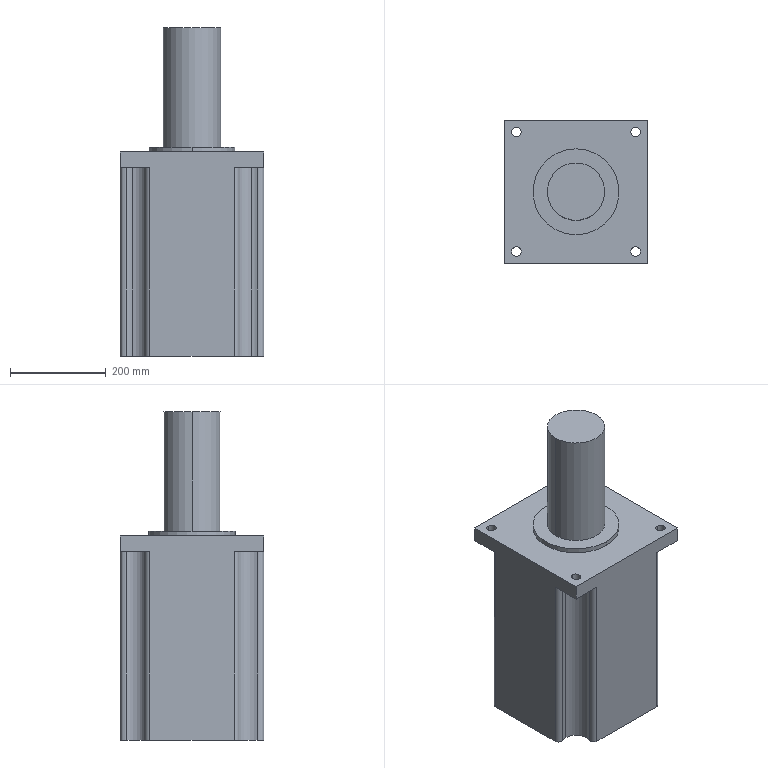Part | SolidWorks | features BaseBody 1, ICE 1, Scale 1 | 1 solid | 40 faces | box 300 x 300 x 687.5 mm | volume 37123455 mm3 | cylinder 28 | plane 12 | commonest cylinder face diameters 20 x18 60 x6 120 x2 180 x2
STEP:
#1=CARTESIAN_POINT('',(2030.017,-675.017,11182.5));
#2=VERTEX_POINT('',#1);
#3=CARTESIAN_POINT('',(1910.017,-675.017,11182.5));
#4=VERTEX_POINT('',#3);
#5=CARTESIAN_POINT('',(1970.017,-675.017,11182.5));
#6=DIRECTION('',(0.,0.,1.));
#7=DIRECTION('',(1.,0.,0.));
#8=AXIS2_PLACEMENT_3D('',#5,#6,#7);
#9=CIRCLE('',#8,60.);
#10=EDGE_CURVE('',#2,#4,#9,.T.);
#11=ORIENTED_EDGE('',*,*,#10,.F.);
#12=CARTESIAN_POINT('',(2030.017,-675.017,10932.5));
#13=VERTEX_POINT('',#12);
#14=CARTESIAN_POINT('',(2030.017,-675.017,11182.5));
#15=DIRECTION('',(0.,0.,-1.));
#16=VECTOR('',#15,1000.);
#17=LINE('',#14,#16);
#18=EDGE_CURVE('',#2,#13,#17,.T.);
#19=ORIENTED_EDGE('',*,*,#18,.T.);
#20=CARTESIAN_POINT('',(1910.017,-675.017,10932.5));
#21=VERTEX_POINT('',#20);
#22=CARTESIAN_POINT('',(1970.017,-675.017,10932.5));
#23=DIRECTION('',(0.,0.,1.));
#24=DIRECTION('',(1.,0.,0.));
#25=AXIS2_PLACEMENT_3D('',#22,#23,#24);
#26=CIRCLE('',#25,60.);
#27=EDGE_CURVE('',#13,#21,#26,.T.);
#28=ORIENTED_EDGE('',*,*,#27,.T.);
#29=CARTESIAN_POINT('',(1910.017,-675.017,11182.5));
#30=DIRECTION('',(0.,0.,-1.));
#31=VECTOR('',#30,1000.);
#32=LINE('',#29,#31);
#33=EDGE_CURVE('',#4,#21,#32,.T.);
#34=ORIENTED_EDGE('',*,*,#33,.F.);
#35=EDGE_LOOP('',(#11,#19,#28,#34));
#36=FACE_OUTER_BOUND('',#35,.T.);
#37=CARTESIAN_POINT('',(1970.017,-675.017,11182.5));
#38=DIRECTION('',(0.,0.,-1.));
#39=DIRECTION('',(-1.,0.,0.));
#40=AXIS2_PLACEMENT_3D('',#37,#38,#39);
#41=CYLINDRICAL_SURFACE('',#40,60.);
#42=ADVANCED_FACE('',(#36),#41,.T.);
#43=CARTESIAN_POINT('',(2106.267,-577.828,10890.));
#44=VERTEX_POINT('',#43);
#45=CARTESIAN_POINT('',(2110.017,-577.098,10890.));
#46=VERTEX_POINT('',#45);
#47=CARTESIAN_POINT('',(2110.017,-587.098,10890.));
#48=DIRECTION('',(0.,0.,-1.));
#49=DIRECTION('',(-1.,0.,0.));
#50=AXIS2_PLACEMENT_3D('',#47,#48,#49);
#51=CIRCLE('',#50,10.);
#52=EDGE_CURVE('',#44,#46,#51,.T.);
#53=ORIENTED_EDGE('',*,*,#52,.T.);
#54=CARTESIAN_POINT('',(2110.017,-577.098,10495.));
#55=VERTEX_POINT('',#54);
#56=CARTESIAN_POINT('',(2110.017,-577.098,10890.));
#57=DIRECTION('',(0.,0.,-1.));
#58=VECTOR('',#57,1000.);
#59=LINE('',#56,#58);
#60=EDGE_CURVE('',#46,#55,#59,.T.);
#61=ORIENTED_EDGE('',*,*,#60,.T.);
#62=CARTESIAN_POINT('',(2106.267,-577.828,10495.));
#63=VERTEX_POINT('',#62);
#64=CARTESIAN_POINT('',(2110.017,-587.098,10495.));
#65=DIRECTION('',(0.,0.,-1.));
#66=DIRECTION('',(-1.,0.,0.));
#67=AXIS2_PLACEMENT_3D('',#64,#65,#66);
#68=CIRCLE('',#67,10.);
#69=EDGE_CURVE('',#63,#55,#68,.T.);
#70=ORIENTED_EDGE('',*,*,#69,.F.);
#71=CARTESIAN_POINT('',(2106.267,-577.828,10890.));
#72=DIRECTION('',(0.,0.,-1.));
#73=VECTOR('',#72,1000.);
#74=LINE('',#71,#73);
#75=EDGE_CURVE('',#44,#63,#74,.T.);
#76=ORIENTED_EDGE('',*,*,#75,.F.);
#77=EDGE_LOOP('',(#53,#61,#70,#76));
#78=FACE_OUTER_BOUND('',#77,.T.);
#79=CARTESIAN_POINT('',(2110.017,-587.098,10890.));
#80=DIRECTION('',(0.,0.,-1.));
#81=DIRECTION('',(0.,1.,0.));
#82=AXIS2_PLACEMENT_3D('',#79,#80,#81);
#83=CYLINDRICAL_SURFACE('',#82,10.);
#84=ADVANCED_FACE('',(#78),#83,.T.);
#85=CARTESIAN_POINT('',(1820.017,-587.098,10890.));
#86=VERTEX_POINT('',#85);
#87=CARTESIAN_POINT('',(1830.017,-577.098,10890.));
#88=VERTEX_POINT('',#87);
#89=CARTESIAN_POINT('',(1830.017,-587.098,10890.));
#90=DIRECTION('',(0.,0.,-1.));
#91=DIRECTION('',(1.,0.,0.));
#92=AXIS2_PLACEMENT_3D('',#89,#90,#91);
#93=CIRCLE('',#92,10.);
#94=EDGE_CURVE('',#86,#88,#93,.T.);
#95=ORIENTED_EDGE('',*,*,#94,.T.);
#96=CARTESIAN_POINT('',(1830.017,-577.098,10495.));
#97=VERTEX_POINT('',#96);
#98=CARTESIAN_POINT('',(1830.017,-577.098,10890.));
#99=DIRECTION('',(0.,0.,-1.));
#100=VECTOR('',#99,1000.);
#101=LINE('',#98,#100);
#102=EDGE_CURVE('',#88,#97,#101,.T.);
#103=ORIENTED_EDGE('',*,*,#102,.T.);
#104=CARTESIAN_POINT('',(1820.017,-587.098,10495.));
#105=VERTEX_POINT('',#104);
#106=CARTESIAN_POINT('',(1830.017,-587.098,10495.));
#107=DIRECTION('',(0.,0.,-1.));
#108=DIRECTION('',(1.,0.,0.));
#109=AXIS2_PLACEMENT_3D('',#106,#107,#108);
#110=CIRCLE('',#109,10.);
#111=EDGE_CURVE('',#105,#97,#110,.T.);
#112=ORIENTED_EDGE('',*,*,#111,.F.);
#113=CARTESIAN_POINT('',(1820.017,-587.098,10890.));
#114=DIRECTION('',(0.,0.,-1.));
#115=VECTOR('',#114,1000.);
#116=LINE('',#113,#115);
#117=EDGE_CURVE('',#86,#105,#116,.T.);
#118=ORIENTED_EDGE('',*,*,#117,.F.);
#119=EDGE_LOOP('',(#95,#103,#112,#118));
#120=FACE_OUTER_BOUND('',#119,.T.);
#121=CARTESIAN_POINT('',(1830.017,-587.098,10890.));
#122=DIRECTION('',(0.,0.,-1.));
#123=DIRECTION('',(0.,1.,0.));
#124=AXIS2_PLACEMENT_3D('',#121,#122,#123);
#125=CYLINDRICAL_SURFACE('',#124,10.);
#126=ADVANCED_FACE('',(#120),#125,.T.);
#127=CARTESIAN_POINT('',(2095.017,-770.017,10890.));
#128=VERTEX_POINT('',#127);
#129=CARTESIAN_POINT('',(2106.267,-772.207,10890.));
#130=VERTEX_POINT('',#129);
#131=CARTESIAN_POINT('',(2095.017,-800.017,10890.));
#132=DIRECTION('',(0.,0.,-1.));
#133=DIRECTION('',(-1.,0.,0.));
#134=AXIS2_PLACEMENT_3D('',#131,#132,#133);
#135=CIRCLE('',#134,30.);
#136=EDGE_CURVE('',#128,#130,#135,.T.);
#137=ORIENTED_EDGE('',*,*,#136,.F.);
#138=CARTESIAN_POINT('',(2095.017,-770.017,10495.));
#139=VERTEX_POINT('',#138);
#140=CARTESIAN_POINT('',(2095.017,-770.017,10890.));
#141=DIRECTION('',(0.,0.,-1.));
#142=VECTOR('',#141,1000.);
#143=LINE('',#140,#142);
#144=EDGE_CURVE('',#128,#139,#143,.T.);
#145=ORIENTED_EDGE('',*,*,#144,.T.);
#146=CARTESIAN_POINT('',(2106.267,-772.207,10495.));
#147=VERTEX_POINT('',#146);
#148=CARTESIAN_POINT('',(2095.017,-800.017,10495.));
#149=DIRECTION('',(0.,0.,-1.));
#150=DIRECTION('',(-1.,0.,0.));
#151=AXIS2_PLACEMENT_3D('',#148,#149,#150);
#152=CIRCLE('',#151,30.);
#153=EDGE_CURVE('',#139,#147,#152,.T.);
#154=ORIENTED_EDGE('',*,*,#153,.T.);
#155=CARTESIAN_POINT('',(2106.267,-772.207,10890.));
#156=DIRECTION('',(0.,0.,-1.));
#157=VECTOR('',#156,1000.);
#158=LINE('',#155,#157);
#159=EDGE_CURVE('',#130,#147,#158,.T.);
#160=ORIENTED_EDGE('',*,*,#159,.F.);
#161=EDGE_LOOP('',(#137,#145,#154,#160));
#162=FACE_OUTER_BOUND('',#161,.T.);
#163=CARTESIAN_POINT('',(2095.017,-800.017,10890.));
#164=DIRECTION('',(0.,0.,-1.));
#165=DIRECTION('',(0.,1.,0.));
#166=AXIS2_PLACEMENT_3D('',#163,#164,#165);
#167=CYLINDRICAL_SURFACE('',#166,30.);
#168=ADVANCED_FACE('',(#162),#167,.F.);
#169=CARTESIAN_POINT('',(1872.828,-811.267,10890.));
#170=VERTEX_POINT('',#169);
#171=CARTESIAN_POINT('',(1845.017,-770.017,10890.));
#172=VERTEX_POINT('',#171);
#173=CARTESIAN_POINT('',(1845.017,-800.017,10890.));
#174=DIRECTION('',(0.,0.,1.));
#175=DIRECTION('',(1.,0.,0.));
#176=AXIS2_PLACEMENT_3D('',#173,#174,#175);
#177=CIRCLE('',#176,30.);
#178=EDGE_CURVE('',#170,#172,#177,.T.);
#179=ORIENTED_EDGE('',*,*,#178,.T.);
#180=CARTESIAN_POINT('',(1845.017,-770.017,10495.));
#181=VERTEX_POINT('',#180);
#182=CARTESIAN_POINT('',(1845.017,-770.017,10890.));
#183=DIRECTION('',(0.,0.,-1.));
#184=VECTOR('',#183,1000.);
#185=LINE('',#182,#184);
#186=EDGE_CURVE('',#172,#181,#185,.T.);
#187=ORIENTED_EDGE('',*,*,#186,.T.);
#188=CARTESIAN_POINT('',(1872.828,-811.267,10495.));
#189=VERTEX_POINT('',#188);
#190=CARTESIAN_POINT('',(1845.017,-800.017,10495.));
#191=DIRECTION('',(0.,0.,1.));
#192=DIRECTION('',(1.,0.,0.));
#193=AXIS2_PLACEMENT_3D('',#190,#191,#192);
#194=CIRCLE('',#193,30.);
#195=EDGE_CURVE('',#189,#181,#194,.T.);
#196=ORIENTED_EDGE('',*,*,#195,.F.);
#197=CARTESIAN_POINT('',(1872.828,-811.267,10890.));
#198=DIRECTION('',(0.,0.,-1.));
#199=VECTOR('',#198,1000.);
#200=LINE('',#197,#199);
#201=EDGE_CURVE('',#170,#189,#200,.T.);
#202=ORIENTED_EDGE('',*,*,#201,.F.);
#203=EDGE_LOOP('',(#179,#187,#196,#202));
#204=FACE_OUTER_BOUND('',#203,.T.);
#205=CARTESIAN_POINT('',(1845.017,-800.017,10890.));
#206=DIRECTION('',(0.,0.,-1.));
#207=DIRECTION('',(0.,1.,0.));
#208=AXIS2_PLACEMENT_3D('',#205,#206,#207);
#209=CYLINDRICAL_SURFACE('',#208,30.);
#210=ADVANCED_FACE('',(#204),#209,.F.);
#211=CARTESIAN_POINT('',(2095.017,-560.017,10922.5));
#212=VERTEX_POINT('',#211);
#213=CARTESIAN_POINT('',(2095.017,-540.017,10922.5));
#214=VERTEX_POINT('',#213);
#215=CARTESIAN_POINT('',(2095.017,-550.017,10922.5));
#216=DIRECTION('',(0.,0.,-1.));
#217=DIRECTION('',(0.,-1.,0.));
#218=AXIS2_PLACEMENT_3D('',#215,#216,#217);
#219=CIRCLE('',#218,10.);
#220=EDGE_CURVE('',#212,#214,#219,.T.);
#221=ORIENTED_EDGE('',*,*,#220,.F.);
#222=CARTESIAN_POINT('',(2095.017,-560.017,10890.));
#223=VERTEX_POINT('',#222);
#224=CARTESIAN_POINT('',(2095.017,-560.017,10995.));
#225=DIRECTION('',(0.,0.,-1.));
#226=VECTOR('',#225,1000.);
#227=LINE('',#224,#226);
#228=EDGE_CURVE('',#212,#223,#227,.T.);
#229=ORIENTED_EDGE('',*,*,#228,.T.);
#230=CARTESIAN_POINT('',(2095.017,-540.017,10890.));
#231=VERTEX_POINT('',#230);
#232=CARTESIAN_POINT('',(2095.017,-550.017,10890.));
#233=DIRECTION('',(0.,0.,1.));
#234=DIRECTION('',(0.,-1.,0.));
#235=AXIS2_PLACEMENT_3D('',#232,#233,#234);
#236=CIRCLE('',#235,10.);
#237=EDGE_CURVE('',#231,#223,#236,.T.);
#238=ORIENTED_EDGE('',*,*,#237,.F.);
#239=CARTESIAN_POINT('',(2095.017,-540.017,10995.));
#240=DIRECTION('',(0.,0.,-1.));
#241=VECTOR('',#240,1000.);
#242=LINE('',#239,#241);
#243=EDGE_CURVE('',#214,#231,#242,.T.);
#244=ORIENTED_EDGE('',*,*,#243,.F.);
#245=EDGE_LOOP('',(#221,#229,#238,#244));
#246=FACE_OUTER_BOUND('',#245,.T.);
#247=CARTESIAN_POINT('',(2095.017,-550.017,10995.));
#248=DIRECTION('',(0.,0.,-1.));
#249=DIRECTION('',(0.,1.,0.));
#250=AXIS2_PLACEMENT_3D('',#247,#248,#249);
#251=CYLINDRICAL_SURFACE('',#250,10.);
#252=ADVANCED_FACE('',(#246),#251,.F.);
#253=CARTESIAN_POINT('',(1970.017,-585.017,10922.5));
#254=VERTEX_POINT('',#253);
#255=CARTESIAN_POINT('',(1970.017,-765.017,10922.5));
#256=VERTEX_POINT('',#255);
#257=CARTESIAN_POINT('',(1970.017,-675.017,10922.5));
#258=DIRECTION('',(0.,0.,1.));
#259=DIRECTION('',(0.,-1.,0.));
#260=AXIS2_PLACEMENT_3D('',#257,#258,#259);
#261=CIRCLE('',#260,90.);
#262=EDGE_CURVE('',#254,#256,#261,.T.);
#263=ORIENTED_EDGE('',*,*,#262,.T.);
#264=CARTESIAN_POINT('',(1970.017,-765.017,10932.5));
#265=VERTEX_POINT('',#264);
#266=CARTESIAN_POINT('',(1970.017,-765.017,10922.5));
#267=DIRECTION('',(0.,0.,1.));
#268=VECTOR('',#267,1000.);
#269=LINE('',#266,#268);
#270=EDGE_CURVE('',#256,#265,#269,.T.);
#271=ORIENTED_EDGE('',*,*,#270,.T.);
#272=CARTESIAN_POINT('',(1970.017,-585.017,10932.5));
#273=VERTEX_POINT('',#272);
#274=CARTESIAN_POINT('',(1970.017,-675.017,10932.5));
#275=DIRECTION('',(0.,0.,-1.));
#276=DIRECTION('',(0.,-1.,0.));
#277=AXIS2_PLACEMENT_3D('',#274,#275,#276);
#278=CIRCLE('',#277,90.);
#279=EDGE_CURVE('',#265,#273,#278,.T.);
#280=ORIENTED_EDGE('',*,*,#279,.T.);
#281=CARTESIAN_POINT('',(1970.017,-585.017,10922.5));
#282=DIRECTION('',(0.,0.,1.));
#283=VECTOR('',#282,1000.);
#284=LINE('',#281,#283);
#285=EDGE_CURVE('',#254,#273,#284,.T.);
#286=ORIENTED_EDGE('',*,*,#285,.F.);
#287=EDGE_LOOP('',(#263,#271,#280,#286));
#288=FACE_OUTER_BOUND('',#287,.T.);
#289=CARTESIAN_POINT('',(1970.017,-675.017,10922.5));
#290=DIRECTION('',(0.,0.,1.));
#291=DIRECTION('',(0.,1.,0.));
#292=AXIS2_PLACEMENT_3D('',#289,#290,#291);
#293=CYLINDRICAL_SURFACE('',#292,90.);
#294=ADVANCED_FACE('',(#288),#293,.T.);
#295=CARTESIAN_POINT('',(1845.017,-810.017,10922.5));
#296=VERTEX_POINT('',#295);
#297=CARTESIAN_POINT('',(1845.017,-790.017,10922.5));
#298=VERTEX_POINT('',#297);
#299=CARTESIAN_POINT('',(1845.017,-800.017,10922.5));
#300=DIRECTION('',(0.,0.,-1.));
#301=DIRECTION('',(0.,-1.,0.));
#302=AXIS2_PLACEMENT_3D('',#299,#300,#301);
#303=CIRCLE('',#302,10.);
#304=EDGE_CURVE('',#296,#298,#303,.T.);
#305=ORIENTED_EDGE('',*,*,#304,.F.);
#306=CARTESIAN_POINT('',(1845.017,-810.017,10890.));
#307=VERTEX_POINT('',#306);
#308=CARTESIAN_POINT('',(1845.017,-810.017,10995.));
#309=DIRECTION('',(0.,0.,-1.));
#310=VECTOR('',#309,1000.);
#311=LINE('',#308,#310);
#312=EDGE_CURVE('',#296,#307,#311,.T.);
#313=ORIENTED_EDGE('',*,*,#312,.T.);
#314=CARTESIAN_POINT('',(1845.017,-790.017,10890.));
#315=VERTEX_POINT('',#314);
#316=CARTESIAN_POINT('',(1845.017,-800.017,10890.));
#317=DIRECTION('',(0.,0.,-1.));
#318=DIRECTION('',(0.,1.,0.));
#319=AXIS2_PLACEMENT_3D('',#316,#317,#318);
#320=CIRCLE('',#319,10.);
#321=EDGE_CURVE('',#307,#315,#320,.T.);
#322=ORIENTED_EDGE('',*,*,#321,.T.);
#323=CARTESIAN_POINT('',(1845.017,-790.017,10995.));
#324=DIRECTION('',(0.,0.,-1.));
#325=VECTOR('',#324,1000.);
#326=LINE('',#323,#325);
#327=EDGE_CURVE('',#298,#315,#326,.T.);
#328=ORIENTED_EDGE('',*,*,#327,.F.);
#329=EDGE_LOOP('',(#305,#313,#322,#328));
#330=FACE_OUTER_BOUND('',#329,.T.);
#331=CARTESIAN_POINT('',(1845.017,-800.017,10995.));
#332=DIRECTION('',(0.,0.,-1.));
#333=DIRECTION('',(0.,1.,0.));
#334=AXIS2_PLACEMENT_3D('',#331,#332,#333);
#335=CYLINDRICAL_SURFACE('',#334,10.);
#336=ADVANCED_FACE('',(#330),#335,.F.);
#337=CARTESIAN_POINT('',(2095.017,-790.017,10922.5));
#338=VERTEX_POINT('',#337);
#339=CARTESIAN_POINT('',(2095.017,-810.017,10922.5));
#340=VERTEX_POINT('',#339);
#341=CARTESIAN_POINT('',(2095.017,-800.017,10922.5));
#342=DIRECTION('',(0.,0.,1.));
#343=DIRECTION('',(0.,-1.,0.));
#344=AXIS2_PLACEMENT_3D('',#341,#342,#343);
#345=CIRCLE('',#344,10.);
#346=EDGE_CURVE('',#338,#340,#345,.T.);
#347=ORIENTED_EDGE('',*,*,#346,.T.);
#348=CARTESIAN_POINT('',(2095.017,-810.017,10890.));
#349=VERTEX_POINT('',#348);
#350=CARTESIAN_POINT('',(2095.017,-810.017,10995.));
#351=DIRECTION('',(0.,0.,-1.));
#352=VECTOR('',#351,1000.);
#353=LINE('',#350,#352);
#354=EDGE_CURVE('',#340,#349,#353,.T.);
#355=ORIENTED_EDGE('',*,*,#354,.T.);
#356=CARTESIAN_POINT('',(2095.017,-790.017,10890.));
#357=VERTEX_POINT('',#356);
#358=CARTESIAN_POINT('',(2095.017,-800.017,10890.));
#359=DIRECTION('',(0.,0.,1.));
#360=DIRECTION('',(0.,1.,0.));
#361=AXIS2_PLACEMENT_3D('',#358,#359,#360);
#362=CIRCLE('',#361,10.);
#363=EDGE_CURVE('',#357,#349,#362,.T.);
#364=ORIENTED_EDGE('',*,*,#363,.F.);
#365=CARTESIAN_POINT('',(2095.017,-790.017,10995.));
#366=DIRECTION('',(0.,0.,-1.));
#367=VECTOR('',#366,1000.);
#368=LINE('',#365,#367);
#369=EDGE_CURVE('',#338,#357,#368,.T.);
#370=ORIENTED_EDGE('',*,*,#369,.F.);
#371=EDGE_LOOP('',(#347,#355,#364,#370));
#372=FACE_OUTER_BOUND('',#371,.T.);
#373=CARTESIAN_POINT('',(2095.017,-800.017,10995.));
#374=DIRECTION('',(0.,0.,-1.));
#375=DIRECTION('',(0.,1.,0.));
#376=AXIS2_PLACEMENT_3D('',#373,#374,#375);
#377=CYLINDRICAL_SURFACE('',#376,10.);
#378=ADVANCED_FACE('',(#372),#377,.F.);
#379=CARTESIAN_POINT('',(1845.017,-560.017,10922.5));
#380=VERTEX_POINT('',#379);
#381=CARTESIAN_POINT('',(1845.017,-540.017,10922.5));
#382=VERTEX_POINT('',#381);
#383=CARTESIAN_POINT('',(1845.017,-550.017,10922.5));
#384=DIRECTION('',(0.,0.,-1.));
#385=DIRECTION('',(0.,-1.,0.));
#386=AXIS2_PLACEMENT_3D('',#383,#384,#385);
#387=CIRCLE('',#386,10.);
#388=EDGE_CURVE('',#380,#382,#387,.T.);
#389=ORIENTED_EDGE('',*,*,#388,.F.);
#390=CARTESIAN_POINT('',(1845.017,-560.017,10890.));
#391=VERTEX_POINT('',#390);
#392=CARTESIAN_POINT('',(1845.017,-560.017,10995.));
#393=DIRECTION('',(0.,0.,-1.));
#394=VECTOR('',#393,1000.);
#395=LINE('',#392,#394);
#396=EDGE_CURVE('',#380,#391,#395,.T.);
#397=ORIENTED_EDGE('',*,*,#396,.T.);
#398=CARTESIAN_POINT('',(1845.017,-540.017,10890.));
#399=VERTEX_POINT('',#398);
#400=CARTESIAN_POINT('',(1845.017,-550.017,10890.));
#401=DIRECTION('',(0.,0.,-1.));
#402=DIRECTION('',(0.,1.,0.));
#403=AXIS2_PLACEMENT_3D('',#400,#401,#402);
#404=CIRCLE('',#403,10.);
#405=EDGE_CURVE('',#391,#399,#404,.T.);
#406=ORIENTED_EDGE('',*,*,#405,.T.);
#407=CARTESIAN_POINT('',(1845.017,-540.017,10995.));
#408=DIRECTION('',(0.,0.,-1.));
#409=VECTOR('',#408,1000.);
#410=LINE('',#407,#409);
#411=EDGE_CURVE('',#382,#399,#410,.T.);
#412=ORIENTED_EDGE('',*,*,#411,.F.);
#413=EDGE_LOOP('',(#389,#397,#406,#412));
#414=FACE_OUTER_BOUND('',#413,.T.);
#415=CARTESIAN_POINT('',(1845.017,-550.017,10995.));
#416=DIRECTION('',(0.,0.,-1.));
#417=DIRECTION('',(0.,1.,0.));
#418=AXIS2_PLACEMENT_3D('',#415,#416,#417);
#419=CYLINDRICAL_SURFACE('',#418,10.);
#420=ADVANCED_FACE('',(#414),#419,.F.);
#421=CARTESIAN_POINT('',(1970.017,-675.017,10932.5));
#422=DIRECTION('',(0.,0.,1.));
#423=DIRECTION('',(1.,0.,0.));
#424=AXIS2_PLACEMENT_3D('',#421,#422,#423);
#425=CIRCLE('',#424,60.);
#426=EDGE_CURVE('',#21,#13,#425,.T.);
#427=ORIENTED_EDGE('',*,*,#426,.F.);
#428=ORIENTED_EDGE('',*,*,#27,.F.);
#429=EDGE_LOOP('',(#427,#428));
#430=FACE_BOUND('',#429,.T.);
#431=CARTESIAN_POINT('',(1970.017,-675.017,10932.5));
#432=DIRECTION('',(0.,0.,-1.));
#433=DIRECTION('',(0.,-1.,0.));
#434=AXIS2_PLACEMENT_3D('',#431,#432,#433);
#435=CIRCLE('',#434,90.);
#436=EDGE_CURVE('',#273,#265,#435,.T.);
#437=ORIENTED_EDGE('',*,*,#436,.F.);
#438=ORIENTED_EDGE('',*,*,#279,.F.);
#439=EDGE_LOOP('',(#437,#438));
#440=FACE_OUTER_BOUND('',#439,.T.);
#441=CARTESIAN_POINT('',(1970.017,-675.017,10932.5));
#442=DIRECTION('',(0.,0.,1.));
#443=DIRECTION('',(0.,1.,0.));
#444=AXIS2_PLACEMENT_3D('',#441,#442,#443);
#445=PLANE('',#444);
#446=ADVANCED_FACE('',(#430,#440),#445,.T.);
#447=CARTESIAN_POINT('',(2067.207,-538.767,10495.));
#448=VERTEX_POINT('',#447);
#449=CARTESIAN_POINT('',(2095.017,-550.017,10495.));
#450=DIRECTION('',(0.,0.,1.));
#451=DIRECTION('',(-1.,0.,0.));
#452=AXIS2_PLACEMENT_3D('',#449,#450,#451);
#453=CIRCLE('',#452,30.);
#454=EDGE_CURVE('',#448,#63,#453,.T.);
#455=ORIENTED_EDGE('',*,*,#454,.T.);
#456=ORIENTED_EDGE('',*,*,#69,.T.);
#457=CARTESIAN_POINT('',(2120.017,-587.098,10495.));
#458=VERTEX_POINT('',#457);
#459=CARTESIAN_POINT('',(2110.017,-587.098,10495.));
#460=DIRECTION('',(0.,0.,-1.));
#461=DIRECTION('',(-1.,0.,0.));
#462=AXIS2_PLACEMENT_3D('',#459,#460,#461);
#463=CIRCLE('',#462,10.);
#464=EDGE_CURVE('',#55,#458,#463,.T.);
#465=ORIENTED_EDGE('',*,*,#464,.T.);
#466=CARTESIAN_POINT('',(2120.017,-762.936,10495.));
#467=VERTEX_POINT('',#466);
#468=CARTESIAN_POINT('',(2120.017,-525.017,10495.));
#469=DIRECTION('',(0.,-1.,0.));
#470=VECTOR('',#469,1000.);
#471=LINE('',#468,#470);
#472=EDGE_CURVE('',#458,#467,#471,.T.);
#473=ORIENTED_EDGE('',*,*,#472,.T.);
#474=CARTESIAN_POINT('',(2110.017,-762.936,10495.));
#475=DIRECTION('',(0.,0.,1.));
#476=DIRECTION('',(-1.,0.,0.));
#477=AXIS2_PLACEMENT_3D('',#474,#475,#476);
#478=CIRCLE('',#477,10.);
#479=EDGE_CURVE('',#147,#467,#478,.T.);
#480=ORIENTED_EDGE('',*,*,#479,.F.);
#481=ORIENTED_EDGE('',*,*,#153,.F.);
#482=CARTESIAN_POINT('',(2067.207,-811.267,10495.));
#483=VERTEX_POINT('',#482);
#484=CARTESIAN_POINT('',(2095.017,-800.017,10495.));
#485=DIRECTION('',(0.,0.,-1.));
#486=DIRECTION('',(-1.,0.,0.));
#487=AXIS2_PLACEMENT_3D('',#484,#485,#486);
#488=CIRCLE('',#487,30.);
#489=EDGE_CURVE('',#483,#139,#488,.T.);
#490=ORIENTED_EDGE('',*,*,#489,.F.);
#491=CARTESIAN_POINT('',(2057.936,-825.017,10495.));
#492=VERTEX_POINT('',#491);
#493=CARTESIAN_POINT('',(2057.936,-815.017,10495.));
#494=DIRECTION('',(0.,0.,1.));
#495=DIRECTION('',(-1.,0.,0.));
#496=AXIS2_PLACEMENT_3D('',#493,#494,#495);
#497=CIRCLE('',#496,10.);
#498=EDGE_CURVE('',#492,#483,#497,.T.);
#499=ORIENTED_EDGE('',*,*,#498,.F.);
#500=CARTESIAN_POINT('',(1882.098,-825.017,10495.));
#501=VERTEX_POINT('',#500);
#502=CARTESIAN_POINT('',(1970.017,-825.017,10495.));
#503=DIRECTION('',(-1.,0.,0.));
#504=VECTOR('',#503,1000.);
#505=LINE('',#502,#504);
#506=EDGE_CURVE('',#492,#501,#505,.T.);
#507=ORIENTED_EDGE('',*,*,#506,.T.);
#508=CARTESIAN_POINT('',(1882.098,-815.017,10495.));
#509=DIRECTION('',(0.,0.,-1.));
#510=DIRECTION('',(1.,0.,0.));
#511=AXIS2_PLACEMENT_3D('',#508,#509,#510);
#512=CIRCLE('',#511,10.);
#513=EDGE_CURVE('',#501,#189,#512,.T.);
#514=ORIENTED_EDGE('',*,*,#513,.T.);
#515=ORIENTED_EDGE('',*,*,#195,.T.);
#516=CARTESIAN_POINT('',(1833.767,-772.207,10495.));
#517=VERTEX_POINT('',#516);
#518=CARTESIAN_POINT('',(1845.017,-800.017,10495.));
#519=DIRECTION('',(0.,0.,1.));
#520=DIRECTION('',(1.,0.,0.));
#521=AXIS2_PLACEMENT_3D('',#518,#519,#520);
#522=CIRCLE('',#521,30.);
#523=EDGE_CURVE('',#181,#517,#522,.T.);
#524=ORIENTED_EDGE('',*,*,#523,.T.);
#525=CARTESIAN_POINT('',(1820.017,-762.936,10495.));
#526=VERTEX_POINT('',#525);
#527=CARTESIAN_POINT('',(1830.017,-762.936,10495.));
#528=DIRECTION('',(0.,0.,-1.));
#529=DIRECTION('',(1.,0.,0.));
#530=AXIS2_PLACEMENT_3D('',#527,#528,#529);
#531=CIRCLE('',#530,10.);
#532=EDGE_CURVE('',#517,#526,#531,.T.);
#533=ORIENTED_EDGE('',*,*,#532,.T.);
#534=CARTESIAN_POINT('',(1820.017,-525.017,10495.));
#535=DIRECTION('',(0.,-1.,0.));
#536=VECTOR('',#535,1000.);
#537=LINE('',#534,#536);
#538=EDGE_CURVE('',#105,#526,#537,.T.);
#539=ORIENTED_EDGE('',*,*,#538,.F.);
#540=ORIENTED_EDGE('',*,*,#111,.T.);
#541=CARTESIAN_POINT('',(1833.767,-577.828,10495.));
#542=VERTEX_POINT('',#541);
#543=CARTESIAN_POINT('',(1830.017,-587.098,10495.));
#544=DIRECTION('',(0.,0.,-1.));
#545=DIRECTION('',(1.,0.,0.));
#546=AXIS2_PLACEMENT_3D('',#543,#544,#545);
#547=CIRCLE('',#546,10.);
#548=EDGE_CURVE('',#97,#542,#547,.T.);
#549=ORIENTED_EDGE('',*,*,#548,.T.);
#550=CARTESIAN_POINT('',(1872.828,-538.767,10495.));
#551=VERTEX_POINT('',#550);
#552=CARTESIAN_POINT('',(1845.017,-550.017,10495.));
#553=DIRECTION('',(0.,0.,1.));
#554=DIRECTION('',(1.,0.,0.));
#555=AXIS2_PLACEMENT_3D('',#552,#553,#554);
#556=CIRCLE('',#555,30.);
#557=EDGE_CURVE('',#542,#551,#556,.T.);
#558=ORIENTED_EDGE('',*,*,#557,.T.);
#559=CARTESIAN_POINT('',(1882.098,-525.017,10495.));
#560=VERTEX_POINT('',#559);
#561=CARTESIAN_POINT('',(1882.098,-535.017,10495.));
#562=DIRECTION('',(0.,0.,-1.));
#563=DIRECTION('',(1.,0.,0.));
#564=AXIS2_PLACEMENT_3D('',#561,#562,#563);
#565=CIRCLE('',#564,10.);
#566=EDGE_CURVE('',#551,#560,#565,.T.);
#567=ORIENTED_EDGE('',*,*,#566,.T.);
#568=CARTESIAN_POINT('',(2057.936,-525.017,10495.));
#569=VERTEX_POINT('',#568);
#570=CARTESIAN_POINT('',(1970.017,-525.017,10495.));
#571=DIRECTION('',(1.,0.,0.));
#572=VECTOR('',#571,1000.);
#573=LINE('',#570,#572);
#574=EDGE_CURVE('',#560,#569,#573,.T.);
#575=ORIENTED_EDGE('',*,*,#574,.T.);
#576=CARTESIAN_POINT('',(2057.936,-535.017,10495.));
#577=DIRECTION('',(0.,0.,-1.));
#578=DIRECTION('',(-1.,0.,0.));
#579=AXIS2_PLACEMENT_3D('',#576,#577,#578);
#580=CIRCLE('',#579,10.);
#581=EDGE_CURVE('',#569,#448,#580,.T.);
#582=ORIENTED_EDGE('',*,*,#581,.T.);
#583=EDGE_LOOP('',(#455,#456,#465,#473,#480,#481,#490,#499,#507,#514,#515,#524,#533,#539,#540,#549,#558,#567,#575,#582));
#584=FACE_OUTER_BOUND('',#583,.T.);
#585=CARTESIAN_POINT('',(1970.017,-525.017,10495.));
#586=DIRECTION('',(0.,0.,-1.));
#587=DIRECTION('',(0.,-1.,0.));
#588=AXIS2_PLACEMENT_3D('',#585,#586,#587);
#589=PLANE('',#588);
#590=ADVANCED_FACE('',(#584),#589,.T.);
#591=CARTESIAN_POINT('',(2120.017,-525.017,10890.));
#592=VERTEX_POINT('',#591);
#593=CARTESIAN_POINT('',(2057.936,-525.017,10890.));
#594=VERTEX_POINT('',#593);
#595=CARTESIAN_POINT('',(2120.017,-525.017,10890.));
#596=DIRECTION('',(-1.,0.,0.));
#597=VECTOR('',#596,1000.);
#598=LINE('',#595,#597);
#599=EDGE_CURVE('',#592,#594,#598,.T.);
#600=ORIENTED_EDGE('',*,*,#599,.T.);
#601=CARTESIAN_POINT('',(2057.936,-525.017,10890.));
#602=DIRECTION('',(0.,0.,-1.));
#603=VECTOR('',#602,1000.);
#604=LINE('',#601,#603);
#605=EDGE_CURVE('',#594,#569,#604,.T.);
#606=ORIENTED_EDGE('',*,*,#605,.T.);
#607=ORIENTED_EDGE('',*,*,#574,.F.);
#608=CARTESIAN_POINT('',(1882.098,-525.017,10890.));
#609=VERTEX_POINT('',#608);
#610=CARTESIAN_POINT('',(1882.098,-525.017,10890.));
#611=DIRECTION('',(0.,0.,-1.));
#612=VECTOR('',#611,1000.);
#613=LINE('',#610,#612);
#614=EDGE_CURVE('',#609,#560,#613,.T.);
#615=ORIENTED_EDGE('',*,*,#614,.F.);
#616=CARTESIAN_POINT('',(1820.017,-525.017,10890.));
#617=VERTEX_POINT('',#616);
#618=CARTESIAN_POINT('',(1882.098,-525.017,10890.));
#619=DIRECTION('',(-1.,0.,0.));
#620=VECTOR('',#619,1000.);
#621=LINE('',#618,#620);
#622=EDGE_CURVE('',#609,#617,#621,.T.);
#623=ORIENTED_EDGE('',*,*,#622,.T.);
#624=CARTESIAN_POINT('',(1820.017,-525.017,10922.5));
#625=VERTEX_POINT('',#624);
#626=CARTESIAN_POINT('',(1820.017,-525.017,10708.75));
#627=DIRECTION('',(0.,0.,-1.));
#628=VECTOR('',#627,1000.);
#629=LINE('',#626,#628);
#630=EDGE_CURVE('',#625,#617,#629,.T.);
#631=ORIENTED_EDGE('',*,*,#630,.F.);
#632=CARTESIAN_POINT('',(2120.017,-525.017,10922.5));
#633=VERTEX_POINT('',#632);
#634=CARTESIAN_POINT('',(1970.017,-525.017,10922.5));
#635=DIRECTION('',(-1.,0.,0.));
#636=VECTOR('',#635,1000.);
#637=LINE('',#634,#636);
#638=EDGE_CURVE('',#633,#625,#637,.T.);
#639=ORIENTED_EDGE('',*,*,#638,.F.);
#640=CARTESIAN_POINT('',(2120.017,-525.017,10708.75));
#641=DIRECTION('',(0.,0.,1.));
#642=VECTOR('',#641,1000.);
#643=LINE('',#640,#642);
#644=EDGE_CURVE('',#592,#633,#643,.T.);
#645=ORIENTED_EDGE('',*,*,#644,.F.);
#646=EDGE_LOOP('',(#600,#606,#607,#615,#623,#631,#639,#645));
#647=FACE_OUTER_BOUND('',#646,.T.);
#648=CARTESIAN_POINT('',(1970.017,-525.017,10708.75));
#649=DIRECTION('',(0.,1.,0.));
#650=DIRECTION('',(1.,0.,0.));
#651=AXIS2_PLACEMENT_3D('',#648,#649,#650);
#652=PLANE('',#651);
#653=ADVANCED_FACE('',(#647),#652,.T.);
#654=CARTESIAN_POINT('',(1820.017,-525.017,10890.));
#655=DIRECTION('',(0.,-1.,0.));
#656=VECTOR('',#655,1000.);
#657=LINE('',#654,#656);
#658=EDGE_CURVE('',#617,#86,#657,.T.);
#659=ORIENTED_EDGE('',*,*,#658,.T.);
#660=ORIENTED_EDGE('',*,*,#117,.T.);
#661=ORIENTED_EDGE('',*,*,#538,.T.);
#662=CARTESIAN_POINT('',(1820.017,-762.936,10890.));
#663=VERTEX_POINT('',#662);
#664=CARTESIAN_POINT('',(1820.017,-762.936,10890.));
#665=DIRECTION('',(0.,0.,-1.));
#666=VECTOR('',#665,1000.);
#667=LINE('',#664,#666);
#668=EDGE_CURVE('',#663,#526,#667,.T.);
#669=ORIENTED_EDGE('',*,*,#668,.F.);
#670=CARTESIAN_POINT('',(1820.017,-825.017,10890.));
#671=VERTEX_POINT('',#670);
#672=CARTESIAN_POINT('',(1820.017,-762.936,10890.));
#673=DIRECTION('',(0.,-1.,0.));
#674=VECTOR('',#673,1000.);
#675=LINE('',#672,#674);
#676=EDGE_CURVE('',#663,#671,#675,.T.);
#677=ORIENTED_EDGE('',*,*,#676,.T.);
#678=CARTESIAN_POINT('',(1820.017,-825.017,10922.5));
#679=VERTEX_POINT('',#678);
#680=CARTESIAN_POINT('',(1820.017,-825.017,10708.75));
#681=DIRECTION('',(0.,0.,1.));
#682=VECTOR('',#681,1000.);
#683=LINE('',#680,#682);
#684=EDGE_CURVE('',#671,#679,#683,.T.);
#685=ORIENTED_EDGE('',*,*,#684,.T.);
#686=CARTESIAN_POINT('',(1820.017,-525.017,10922.5));
#687=DIRECTION('',(0.,-1.,0.));
#688=VECTOR('',#687,1000.);
#689=LINE('',#686,#688);
#690=EDGE_CURVE('',#625,#679,#689,.T.);
#691=ORIENTED_EDGE('',*,*,#690,.F.);
#692=ORIENTED_EDGE('',*,*,#630,.T.);
#693=EDGE_LOOP('',(#659,#660,#661,#669,#677,#685,#691,#692));
#694=FACE_OUTER_BOUND('',#693,.T.);
#695=CARTESIAN_POINT('',(1820.017,-525.017,10708.75));
#696=DIRECTION('',(-1.,0.,0.));
#697=DIRECTION('',(0.,1.,0.));
#698=AXIS2_PLACEMENT_3D('',#695,#696,#697);
#699=PLANE('',#698);
#700=ADVANCED_FACE('',(#694),#699,.T.);
#701=ORIENTED_EDGE('',*,*,#396,.F.);
#702=CARTESIAN_POINT('',(1845.017,-550.017,10922.5));
#703=DIRECTION('',(0.,0.,-1.));
#704=DIRECTION('',(0.,-1.,0.));
#705=AXIS2_PLACEMENT_3D('',#702,#703,#704);
#706=CIRCLE('',#705,10.);
#707=EDGE_CURVE('',#382,#380,#706,.T.);
#708=ORIENTED_EDGE('',*,*,#707,.F.);
#709=ORIENTED_EDGE('',*,*,#411,.T.);
#710=CARTESIAN_POINT('',(1845.017,-550.017,10890.));
#711=DIRECTION('',(0.,0.,-1.));
#712=DIRECTION('',(0.,1.,0.));
#713=AXIS2_PLACEMENT_3D('',#710,#711,#712);
#714=CIRCLE('',#713,10.);
#715=EDGE_CURVE('',#399,#391,#714,.T.);
#716=ORIENTED_EDGE('',*,*,#715,.T.);
#717=EDGE_LOOP('',(#701,#708,#709,#716));
#718=FACE_OUTER_BOUND('',#717,.T.);
#719=CARTESIAN_POINT('',(1845.017,-550.017,10995.));
#720=DIRECTION('',(0.,0.,-1.));
#721=DIRECTION('',(0.,1.,0.));
#722=AXIS2_PLACEMENT_3D('',#719,#720,#721);
#723=CYLINDRICAL_SURFACE('',#722,10.);
#724=ADVANCED_FACE('',(#718),#723,.F.);
#725=ORIENTED_EDGE('',*,*,#506,.F.);
#726=CARTESIAN_POINT('',(2057.936,-825.017,10890.));
#727=VERTEX_POINT('',#726);
#728=CARTESIAN_POINT('',(2057.936,-825.017,10890.));
#729=DIRECTION('',(0.,0.,-1.));
#730=VECTOR('',#729,1000.);
#731=LINE('',#728,#730);
#732=EDGE_CURVE('',#727,#492,#731,.T.);
#733=ORIENTED_EDGE('',*,*,#732,.F.);
#734=CARTESIAN_POINT('',(2120.017,-825.017,10890.));
#735=VERTEX_POINT('',#734);
#736=CARTESIAN_POINT('',(2120.017,-825.017,10890.));
#737=DIRECTION('',(-1.,0.,0.));
#738=VECTOR('',#737,1000.);
#739=LINE('',#736,#738);
#740=EDGE_CURVE('',#735,#727,#739,.T.);
#741=ORIENTED_EDGE('',*,*,#740,.F.);
#742=CARTESIAN_POINT('',(2120.017,-825.017,10922.5));
#743=VERTEX_POINT('',#742);
#744=CARTESIAN_POINT('',(2120.017,-825.017,10708.75));
#745=DIRECTION('',(0.,0.,-1.));
#746=VECTOR('',#745,1000.);
#747=LINE('',#744,#746);
#748=EDGE_CURVE('',#743,#735,#747,.T.);
#749=ORIENTED_EDGE('',*,*,#748,.F.);
#750=CARTESIAN_POINT('',(1970.017,-825.017,10922.5));
#751=DIRECTION('',(1.,0.,0.));
#752=VECTOR('',#751,1000.);
#753=LINE('',#750,#752);
#754=EDGE_CURVE('',#679,#743,#753,.T.);
#755=ORIENTED_EDGE('',*,*,#754,.F.);
#756=ORIENTED_EDGE('',*,*,#684,.F.);
#757=CARTESIAN_POINT('',(1882.098,-825.017,10890.));
#758=VERTEX_POINT('',#757);
#759=CARTESIAN_POINT('',(1820.017,-825.017,10890.));
#760=DIRECTION('',(1.,0.,0.));
#761=VECTOR('',#760,1000.);
#762=LINE('',#759,#761);
#763=EDGE_CURVE('',#671,#758,#762,.T.);
#764=ORIENTED_EDGE('',*,*,#763,.T.);
#765=CARTESIAN_POINT('',(1882.098,-825.017,10890.));
#766=DIRECTION('',(0.,0.,-1.));
#767=VECTOR('',#766,1000.);
#768=LINE('',#765,#767);
#769=EDGE_CURVE('',#758,#501,#768,.T.);
#770=ORIENTED_EDGE('',*,*,#769,.T.);
#771=EDGE_LOOP('',(#725,#733,#741,#749,#755,#756,#764,#770));
#772=FACE_OUTER_BOUND('',#771,.T.);
#773=CARTESIAN_POINT('',(1970.017,-825.017,10708.75));
#774=DIRECTION('',(0.,-1.,0.));
#775=DIRECTION('',(-1.,0.,0.));
#776=AXIS2_PLACEMENT_3D('',#773,#774,#775);
#777=PLANE('',#776);
#778=ADVANCED_FACE('',(#772),#777,.T.);
#779=ORIENTED_EDGE('',*,*,#354,.F.);
#780=CARTESIAN_POINT('',(2095.017,-800.017,10922.5));
#781=DIRECTION('',(0.,0.,1.));
#782=DIRECTION('',(0.,-1.,0.));
#783=AXIS2_PLACEMENT_3D('',#780,#781,#782);
#784=CIRCLE('',#783,10.);
#785=EDGE_CURVE('',#340,#338,#784,.T.);
#786=ORIENTED_EDGE('',*,*,#785,.T.);
#787=ORIENTED_EDGE('',*,*,#369,.T.);
#788=CARTESIAN_POINT('',(2095.017,-800.017,10890.));
#789=DIRECTION('',(0.,0.,1.));
#790=DIRECTION('',(0.,1.,0.));
#791=AXIS2_PLACEMENT_3D('',#788,#789,#790);
#792=CIRCLE('',#791,10.);
#793=EDGE_CURVE('',#349,#357,#792,.T.);
#794=ORIENTED_EDGE('',*,*,#793,.F.);
#795=EDGE_LOOP('',(#779,#786,#787,#794));
#796=FACE_OUTER_BOUND('',#795,.T.);
#797=CARTESIAN_POINT('',(2095.017,-800.017,10995.));
#798=DIRECTION('',(0.,0.,-1.));
#799=DIRECTION('',(0.,1.,0.));
#800=AXIS2_PLACEMENT_3D('',#797,#798,#799);
#801=CYLINDRICAL_SURFACE('',#800,10.);
#802=ADVANCED_FACE('',(#796),#801,.F.);
#803=ORIENTED_EDGE('',*,*,#312,.F.);
#804=CARTESIAN_POINT('',(1845.017,-800.017,10922.5));
#805=DIRECTION('',(0.,0.,-1.));
#806=DIRECTION('',(0.,-1.,0.));
#807=AXIS2_PLACEMENT_3D('',#804,#805,#806);
#808=CIRCLE('',#807,10.);
#809=EDGE_CURVE('',#298,#296,#808,.T.);
#810=ORIENTED_EDGE('',*,*,#809,.F.);
#811=ORIENTED_EDGE('',*,*,#327,.T.);
#812=CARTESIAN_POINT('',(1845.017,-800.017,10890.));
#813=DIRECTION('',(0.,0.,-1.));
#814=DIRECTION('',(0.,1.,0.));
#815=AXIS2_PLACEMENT_3D('',#812,#813,#814);
#816=CIRCLE('',#815,10.);
#817=EDGE_CURVE('',#315,#307,#816,.T.);
#818=ORIENTED_EDGE('',*,*,#817,.T.);
#819=EDGE_LOOP('',(#803,#810,#811,#818));
#820=FACE_OUTER_BOUND('',#819,.T.);
#821=CARTESIAN_POINT('',(1845.017,-800.017,10995.));
#822=DIRECTION('',(0.,0.,-1.));
#823=DIRECTION('',(0.,1.,0.));
#824=AXIS2_PLACEMENT_3D('',#821,#822,#823);
#825=CYLINDRICAL_SURFACE('',#824,10.);
#826=ADVANCED_FACE('',(#820),#825,.F.);
#827=ORIENTED_EDGE('',*,*,#809,.T.);
#828=ORIENTED_EDGE('',*,*,#304,.T.);
#829=EDGE_LOOP('',(#827,#828));
#830=FACE_BOUND('',#829,.T.);
#831=ORIENTED_EDGE('',*,*,#346,.F.);
#832=ORIENTED_EDGE('',*,*,#785,.F.);
#833=EDGE_LOOP('',(#831,#832));
#834=FACE_BOUND('',#833,.T.);
#835=ORIENTED_EDGE('',*,*,#690,.T.);
#836=ORIENTED_EDGE('',*,*,#754,.T.);
#837=CARTESIAN_POINT('',(2120.017,-525.017,10922.5));
#838=DIRECTION('',(0.,-1.,0.));
#839=VECTOR('',#838,1000.);
#840=LINE('',#837,#839);
#841=EDGE_CURVE('',#633,#743,#840,.T.);
#842=ORIENTED_EDGE('',*,*,#841,.F.);
#843=ORIENTED_EDGE('',*,*,#638,.T.);
#844=EDGE_LOOP('',(#835,#836,#842,#843));
#845=FACE_OUTER_BOUND('',#844,.T.);
#846=ORIENTED_EDGE('',*,*,#262,.F.);
#847=CARTESIAN_POINT('',(1970.017,-675.017,10922.5));
#848=DIRECTION('',(0.,0.,1.));
#849=DIRECTION('',(0.,-1.,0.));
#850=AXIS2_PLACEMENT_3D('',#847,#848,#849);
#851=CIRCLE('',#850,90.);
#852=EDGE_CURVE('',#256,#254,#851,.T.);
#853=ORIENTED_EDGE('',*,*,#852,.F.);
#854=EDGE_LOOP('',(#846,#853));
#855=FACE_BOUND('',#854,.T.);
#856=CARTESIAN_POINT('',(2095.017,-550.017,10922.5));
#857=DIRECTION('',(0.,0.,-1.));
#858=DIRECTION('',(0.,-1.,0.));
#859=AXIS2_PLACEMENT_3D('',#856,#857,#858);
#860=CIRCLE('',#859,10.);
#861=EDGE_CURVE('',#214,#212,#860,.T.);
#862=ORIENTED_EDGE('',*,*,#861,.T.);
#863=ORIENTED_EDGE('',*,*,#220,.T.);
#864=EDGE_LOOP('',(#862,#863));
#865=FACE_BOUND('',#864,.T.);
#866=ORIENTED_EDGE('',*,*,#707,.T.);
#867=ORIENTED_EDGE('',*,*,#388,.T.);
#868=EDGE_LOOP('',(#866,#867));
#869=FACE_BOUND('',#868,.T.);
#870=CARTESIAN_POINT('',(1970.017,-525.017,10922.5));
#871=DIRECTION('',(0.,0.,1.));
#872=DIRECTION('',(0.,1.,0.));
#873=AXIS2_PLACEMENT_3D('',#870,#871,#872);
#874=PLANE('',#873);
#875=ADVANCED_FACE('',(#830,#834,#845,#855,#865,#869),#874,.T.);
#876=CARTESIAN_POINT('',(2120.017,-587.098,10890.));
#877=VERTEX_POINT('',#876);
#878=CARTESIAN_POINT('',(2120.017,-587.098,10890.));
#879=DIRECTION('',(0.,0.,-1.));
#880=VECTOR('',#879,1000.);
#881=LINE('',#878,#880);
#882=EDGE_CURVE('',#877,#458,#881,.T.);
#883=ORIENTED_EDGE('',*,*,#882,.F.);
#884=CARTESIAN_POINT('',(2120.017,-587.098,10890.));
#885=DIRECTION('',(0.,1.,0.));
#886=VECTOR('',#885,1000.);
#887=LINE('',#884,#886);
#888=EDGE_CURVE('',#877,#592,#887,.T.);
#889=ORIENTED_EDGE('',*,*,#888,.T.);
#890=ORIENTED_EDGE('',*,*,#644,.T.);
#891=ORIENTED_EDGE('',*,*,#841,.T.);
#892=ORIENTED_EDGE('',*,*,#748,.T.);
#893=CARTESIAN_POINT('',(2120.017,-762.936,10890.));
#894=VERTEX_POINT('',#893);
#895=CARTESIAN_POINT('',(2120.017,-762.936,10890.));
#896=DIRECTION('',(0.,-1.,0.));
#897=VECTOR('',#896,1000.);
#898=LINE('',#895,#897);
#899=EDGE_CURVE('',#894,#735,#898,.T.);
#900=ORIENTED_EDGE('',*,*,#899,.F.);
#901=CARTESIAN_POINT('',(2120.017,-762.936,10890.));
#902=DIRECTION('',(0.,0.,-1.));
#903=VECTOR('',#902,1000.);
#904=LINE('',#901,#903);
#905=EDGE_CURVE('',#894,#467,#904,.T.);
#906=ORIENTED_EDGE('',*,*,#905,.T.);
#907=ORIENTED_EDGE('',*,*,#472,.F.);
#908=EDGE_LOOP('',(#883,#889,#890,#891,#892,#900,#906,#907));
#909=FACE_OUTER_BOUND('',#908,.T.);
#910=CARTESIAN_POINT('',(2120.017,-525.017,10708.75));
#911=DIRECTION('',(1.,0.,0.));
#912=DIRECTION('',(0.,-1.,0.));
#913=AXIS2_PLACEMENT_3D('',#910,#911,#912);
#914=PLANE('',#913);
#915=ADVANCED_FACE('',(#909),#914,.T.);
#916=ORIENTED_EDGE('',*,*,#270,.F.);
#917=ORIENTED_EDGE('',*,*,#852,.T.);
#918=ORIENTED_EDGE('',*,*,#285,.T.);
#919=ORIENTED_EDGE('',*,*,#436,.T.);
#920=EDGE_LOOP('',(#916,#917,#918,#919));
#921=FACE_OUTER_BOUND('',#920,.T.);
#922=CARTESIAN_POINT('',(1970.017,-675.017,10922.5));
#923=DIRECTION('',(0.,0.,1.));
#924=DIRECTION('',(0.,1.,0.));
#925=AXIS2_PLACEMENT_3D('',#922,#923,#924);
#926=CYLINDRICAL_SURFACE('',#925,90.);
#927=ADVANCED_FACE('',(#921),#926,.T.);
#928=ORIENTED_EDGE('',*,*,#228,.F.);
#929=ORIENTED_EDGE('',*,*,#861,.F.);
#930=ORIENTED_EDGE('',*,*,#243,.T.);
#931=CARTESIAN_POINT('',(2095.017,-550.017,10890.));
#932=DIRECTION('',(0.,0.,1.));
#933=DIRECTION('',(0.,-1.,0.));
#934=AXIS2_PLACEMENT_3D('',#931,#932,#933);
#935=CIRCLE('',#934,10.);
#936=EDGE_CURVE('',#223,#231,#935,.T.);
#937=ORIENTED_EDGE('',*,*,#936,.F.);
#938=EDGE_LOOP('',(#928,#929,#930,#937));
#939=FACE_OUTER_BOUND('',#938,.T.);
#940=CARTESIAN_POINT('',(2095.017,-550.017,10995.));
#941=DIRECTION('',(0.,0.,-1.));
#942=DIRECTION('',(0.,1.,0.));
#943=AXIS2_PLACEMENT_3D('',#940,#941,#942);
#944=CYLINDRICAL_SURFACE('',#943,10.);
#945=ADVANCED_FACE('',(#939),#944,.F.);
#946=ORIENTED_EDGE('',*,*,#532,.F.);
#947=CARTESIAN_POINT('',(1833.767,-772.207,10890.));
#948=VERTEX_POINT('',#947);
#949=CARTESIAN_POINT('',(1833.767,-772.207,10890.));
#950=DIRECTION('',(0.,0.,-1.));
#951=VECTOR('',#950,1000.);
#952=LINE('',#949,#951);
#953=EDGE_CURVE('',#948,#517,#952,.T.);
#954=ORIENTED_EDGE('',*,*,#953,.F.);
#955=CARTESIAN_POINT('',(1830.017,-762.936,10890.));
#956=DIRECTION('',(0.,0.,-1.));
#957=DIRECTION('',(1.,0.,0.));
#958=AXIS2_PLACEMENT_3D('',#955,#956,#957);
#959=CIRCLE('',#958,10.);
#960=EDGE_CURVE('',#948,#663,#959,.T.);
#961=ORIENTED_EDGE('',*,*,#960,.T.);
#962=ORIENTED_EDGE('',*,*,#668,.T.);
#963=EDGE_LOOP('',(#946,#954,#961,#962));
#964=FACE_OUTER_BOUND('',#963,.T.);
#965=CARTESIAN_POINT('',(1830.017,-762.936,10890.));
#966=DIRECTION('',(0.,0.,-1.));
#967=DIRECTION('',(0.,1.,0.));
#968=AXIS2_PLACEMENT_3D('',#965,#966,#967);
#969=CYLINDRICAL_SURFACE('',#968,10.);
#970=ADVANCED_FACE('',(#964),#969,.T.);
#971=ORIENTED_EDGE('',*,*,#513,.F.);
#972=ORIENTED_EDGE('',*,*,#769,.F.);
#973=CARTESIAN_POINT('',(1882.098,-815.017,10890.));
#974=DIRECTION('',(0.,0.,-1.));
#975=DIRECTION('',(1.,0.,0.));
#976=AXIS2_PLACEMENT_3D('',#973,#974,#975);
#977=CIRCLE('',#976,10.);
#978=EDGE_CURVE('',#758,#170,#977,.T.);
#979=ORIENTED_EDGE('',*,*,#978,.T.);
#980=ORIENTED_EDGE('',*,*,#201,.T.);
#981=EDGE_LOOP('',(#971,#972,#979,#980));
#982=FACE_OUTER_BOUND('',#981,.T.);
#983=CARTESIAN_POINT('',(1882.098,-815.017,10890.));
#984=DIRECTION('',(0.,0.,-1.));
#985=DIRECTION('',(0.,1.,0.));
#986=AXIS2_PLACEMENT_3D('',#983,#984,#985);
#987=CYLINDRICAL_SURFACE('',#986,10.);
#988=ADVANCED_FACE('',(#982),#987,.T.);
#989=ORIENTED_EDGE('',*,*,#186,.F.);
#990=CARTESIAN_POINT('',(1845.017,-800.017,10890.));
#991=DIRECTION('',(0.,0.,1.));
#992=DIRECTION('',(1.,0.,0.));
#993=AXIS2_PLACEMENT_3D('',#990,#991,#992);
#994=CIRCLE('',#993,30.);
#995=EDGE_CURVE('',#172,#948,#994,.T.);
#996=ORIENTED_EDGE('',*,*,#995,.T.);
#997=ORIENTED_EDGE('',*,*,#953,.T.);
#998=ORIENTED_EDGE('',*,*,#523,.F.);
#999=EDGE_LOOP('',(#989,#996,#997,#998));
#1000=FACE_OUTER_BOUND('',#999,.T.);
#1001=CARTESIAN_POINT('',(1845.017,-800.017,10890.));
#1002=DIRECTION('',(0.,0.,-1.));
#1003=DIRECTION('',(0.,1.,0.));
#1004=AXIS2_PLACEMENT_3D('',#1001,#1002,#1003);
#1005=CYLINDRICAL_SURFACE('',#1004,30.);
#1006=ADVANCED_FACE('',(#1000),#1005,.F.);
#1007=ORIENTED_EDGE('',*,*,#817,.F.);
#1008=ORIENTED_EDGE('',*,*,#321,.F.);
#1009=EDGE_LOOP('',(#1007,#1008));
#1010=FACE_BOUND('',#1009,.T.);
#1011=ORIENTED_EDGE('',*,*,#960,.F.);
#1012=ORIENTED_EDGE('',*,*,#995,.F.);
#1013=ORIENTED_EDGE('',*,*,#178,.F.);
#1014=ORIENTED_EDGE('',*,*,#978,.F.);
#1015=ORIENTED_EDGE('',*,*,#763,.F.);
#1016=ORIENTED_EDGE('',*,*,#676,.F.);
#1017=EDGE_LOOP('',(#1011,#1012,#1013,#1014,#1015,#1016));
#1018=FACE_OUTER_BOUND('',#1017,.T.);
#1019=CARTESIAN_POINT('',(1830.017,-762.936,10890.));
#1020=DIRECTION('',(0.,0.,-1.));
#1021=DIRECTION('',(0.,1.,0.));
#1022=AXIS2_PLACEMENT_3D('',#1019,#1020,#1021);
#1023=PLANE('',#1022);
#1024=ADVANCED_FACE('',(#1010,#1018),#1023,.T.);
#1025=CARTESIAN_POINT('',(2067.207,-811.267,10890.));
#1026=VERTEX_POINT('',#1025);
#1027=CARTESIAN_POINT('',(2095.017,-800.017,10890.));
#1028=DIRECTION('',(0.,0.,-1.));
#1029=DIRECTION('',(-1.,0.,0.));
#1030=AXIS2_PLACEMENT_3D('',#1027,#1028,#1029);
#1031=CIRCLE('',#1030,30.);
#1032=EDGE_CURVE('',#1026,#128,#1031,.T.);
#1033=ORIENTED_EDGE('',*,*,#1032,.T.);
#1034=ORIENTED_EDGE('',*,*,#136,.T.);
#1035=CARTESIAN_POINT('',(2110.017,-762.936,10890.));
#1036=DIRECTION('',(0.,0.,1.));
#1037=DIRECTION('',(-1.,0.,0.));
#1038=AXIS2_PLACEMENT_3D('',#1035,#1036,#1037);
#1039=CIRCLE('',#1038,10.);
#1040=EDGE_CURVE('',#130,#894,#1039,.T.);
#1041=ORIENTED_EDGE('',*,*,#1040,.T.);
#1042=ORIENTED_EDGE('',*,*,#899,.T.);
#1043=ORIENTED_EDGE('',*,*,#740,.T.);
#1044=CARTESIAN_POINT('',(2057.936,-815.017,10890.));
#1045=DIRECTION('',(0.,0.,1.));
#1046=DIRECTION('',(-1.,0.,0.));
#1047=AXIS2_PLACEMENT_3D('',#1044,#1045,#1046);
#1048=CIRCLE('',#1047,10.);
#1049=EDGE_CURVE('',#727,#1026,#1048,.T.);
#1050=ORIENTED_EDGE('',*,*,#1049,.T.);
#1051=EDGE_LOOP('',(#1033,#1034,#1041,#1042,#1043,#1050));
#1052=FACE_OUTER_BOUND('',#1051,.T.);
#1053=ORIENTED_EDGE('',*,*,#363,.T.);
#1054=ORIENTED_EDGE('',*,*,#793,.T.);
#1055=EDGE_LOOP('',(#1053,#1054));
#1056=FACE_BOUND('',#1055,.T.);
#1057=CARTESIAN_POINT('',(2095.017,-800.017,10890.));
#1058=DIRECTION('',(0.,0.,-1.));
#1059=DIRECTION('',(0.,1.,0.));
#1060=AXIS2_PLACEMENT_3D('',#1057,#1058,#1059);
#1061=PLANE('',#1060);
#1062=ADVANCED_FACE('',(#1052,#1056),#1061,.T.);
#1063=ORIENTED_EDGE('',*,*,#479,.T.);
#1064=ORIENTED_EDGE('',*,*,#905,.F.);
#1065=ORIENTED_EDGE('',*,*,#1040,.F.);
#1066=ORIENTED_EDGE('',*,*,#159,.T.);
#1067=EDGE_LOOP('',(#1063,#1064,#1065,#1066));
#1068=FACE_OUTER_BOUND('',#1067,.T.);
#1069=CARTESIAN_POINT('',(2110.017,-762.936,10890.));
#1070=DIRECTION('',(0.,0.,-1.));
#1071=DIRECTION('',(0.,1.,0.));
#1072=AXIS2_PLACEMENT_3D('',#1069,#1070,#1071);
#1073=CYLINDRICAL_SURFACE('',#1072,10.);
#1074=ADVANCED_FACE('',(#1068),#1073,.T.);
#1075=ORIENTED_EDGE('',*,*,#498,.T.);
#1076=CARTESIAN_POINT('',(2067.207,-811.267,10890.));
#1077=DIRECTION('',(0.,0.,-1.));
#1078=VECTOR('',#1077,1000.);
#1079=LINE('',#1076,#1078);
#1080=EDGE_CURVE('',#1026,#483,#1079,.T.);
#1081=ORIENTED_EDGE('',*,*,#1080,.F.);
#1082=ORIENTED_EDGE('',*,*,#1049,.F.);
#1083=ORIENTED_EDGE('',*,*,#732,.T.);
#1084=EDGE_LOOP('',(#1075,#1081,#1082,#1083));
#1085=FACE_OUTER_BOUND('',#1084,.T.);
#1086=CARTESIAN_POINT('',(2057.936,-815.017,10890.));
#1087=DIRECTION('',(0.,0.,-1.));
#1088=DIRECTION('',(0.,1.,0.));
#1089=AXIS2_PLACEMENT_3D('',#1086,#1087,#1088);
#1090=CYLINDRICAL_SURFACE('',#1089,10.);
#1091=ADVANCED_FACE('',(#1085),#1090,.T.);
#1092=ORIENTED_EDGE('',*,*,#144,.F.);
#1093=ORIENTED_EDGE('',*,*,#1032,.F.);
#1094=ORIENTED_EDGE('',*,*,#1080,.T.);
#1095=ORIENTED_EDGE('',*,*,#489,.T.);
#1096=EDGE_LOOP('',(#1092,#1093,#1094,#1095));
#1097=FACE_OUTER_BOUND('',#1096,.T.);
#1098=CARTESIAN_POINT('',(2095.017,-800.017,10890.));
#1099=DIRECTION('',(0.,0.,-1.));
#1100=DIRECTION('',(0.,1.,0.));
#1101=AXIS2_PLACEMENT_3D('',#1098,#1099,#1100);
#1102=CYLINDRICAL_SURFACE('',#1101,30.);
#1103=ADVANCED_FACE('',(#1097),#1102,.F.);
#1104=ORIENTED_EDGE('',*,*,#102,.F.);
#1105=CARTESIAN_POINT('',(1833.767,-577.828,10890.));
#1106=VERTEX_POINT('',#1105);
#1107=CARTESIAN_POINT('',(1830.017,-587.098,10890.));
#1108=DIRECTION('',(0.,0.,-1.));
#1109=DIRECTION('',(1.,0.,0.));
#1110=AXIS2_PLACEMENT_3D('',#1107,#1108,#1109);
#1111=CIRCLE('',#1110,10.);
#1112=EDGE_CURVE('',#88,#1106,#1111,.T.);
#1113=ORIENTED_EDGE('',*,*,#1112,.T.);
#1114=CARTESIAN_POINT('',(1833.767,-577.828,10890.));
#1115=DIRECTION('',(0.,0.,-1.));
#1116=VECTOR('',#1115,1000.);
#1117=LINE('',#1114,#1116);
#1118=EDGE_CURVE('',#1106,#542,#1117,.T.);
#1119=ORIENTED_EDGE('',*,*,#1118,.T.);
#1120=ORIENTED_EDGE('',*,*,#548,.F.);
#1121=EDGE_LOOP('',(#1104,#1113,#1119,#1120));
#1122=FACE_OUTER_BOUND('',#1121,.T.);
#1123=CARTESIAN_POINT('',(1830.017,-587.098,10890.));
#1124=DIRECTION('',(0.,0.,-1.));
#1125=DIRECTION('',(0.,1.,0.));
#1126=AXIS2_PLACEMENT_3D('',#1123,#1124,#1125);
#1127=CYLINDRICAL_SURFACE('',#1126,10.);
#1128=ADVANCED_FACE('',(#1122),#1127,.T.);
#1129=ORIENTED_EDGE('',*,*,#557,.F.);
#1130=ORIENTED_EDGE('',*,*,#1118,.F.);
#1131=CARTESIAN_POINT('',(1872.828,-538.767,10890.));
#1132=VERTEX_POINT('',#1131);
#1133=CARTESIAN_POINT('',(1845.017,-550.017,10890.));
#1134=DIRECTION('',(0.,0.,1.));
#1135=DIRECTION('',(1.,0.,0.));
#1136=AXIS2_PLACEMENT_3D('',#1133,#1134,#1135);
#1137=CIRCLE('',#1136,30.);
#1138=EDGE_CURVE('',#1106,#1132,#1137,.T.);
#1139=ORIENTED_EDGE('',*,*,#1138,.T.);
#1140=CARTESIAN_POINT('',(1872.828,-538.767,10890.));
#1141=DIRECTION('',(0.,0.,-1.));
#1142=VECTOR('',#1141,1000.);
#1143=LINE('',#1140,#1142);
#1144=EDGE_CURVE('',#1132,#551,#1143,.T.);
#1145=ORIENTED_EDGE('',*,*,#1144,.T.);
#1146=EDGE_LOOP('',(#1129,#1130,#1139,#1145));
#1147=FACE_OUTER_BOUND('',#1146,.T.);
#1148=CARTESIAN_POINT('',(1845.017,-550.017,10890.));
#1149=DIRECTION('',(0.,0.,-1.));
#1150=DIRECTION('',(0.,1.,0.));
#1151=AXIS2_PLACEMENT_3D('',#1148,#1149,#1150);
#1152=CYLINDRICAL_SURFACE('',#1151,30.);
#1153=ADVANCED_FACE('',(#1147),#1152,.F.);
#1154=ORIENTED_EDGE('',*,*,#566,.F.);
#1155=ORIENTED_EDGE('',*,*,#1144,.F.);
#1156=CARTESIAN_POINT('',(1882.098,-535.017,10890.));
#1157=DIRECTION('',(0.,0.,-1.));
#1158=DIRECTION('',(1.,0.,0.));
#1159=AXIS2_PLACEMENT_3D('',#1156,#1157,#1158);
#1160=CIRCLE('',#1159,10.);
#1161=EDGE_CURVE('',#1132,#609,#1160,.T.);
#1162=ORIENTED_EDGE('',*,*,#1161,.T.);
#1163=ORIENTED_EDGE('',*,*,#614,.T.);
#1164=EDGE_LOOP('',(#1154,#1155,#1162,#1163));
#1165=FACE_OUTER_BOUND('',#1164,.T.);
#1166=CARTESIAN_POINT('',(1882.098,-535.017,10890.));
#1167=DIRECTION('',(0.,0.,-1.));
#1168=DIRECTION('',(0.,1.,0.));
#1169=AXIS2_PLACEMENT_3D('',#1166,#1167,#1168);
#1170=CYLINDRICAL_SURFACE('',#1169,10.);
#1171=ADVANCED_FACE('',(#1165),#1170,.T.);
#1172=ORIENTED_EDGE('',*,*,#715,.F.);
#1173=ORIENTED_EDGE('',*,*,#405,.F.);
#1174=EDGE_LOOP('',(#1172,#1173));
#1175=FACE_BOUND('',#1174,.T.);
#1176=ORIENTED_EDGE('',*,*,#658,.F.);
#1177=ORIENTED_EDGE('',*,*,#622,.F.);
#1178=ORIENTED_EDGE('',*,*,#1161,.F.);
#1179=ORIENTED_EDGE('',*,*,#1138,.F.);
#1180=ORIENTED_EDGE('',*,*,#1112,.F.);
#1181=ORIENTED_EDGE('',*,*,#94,.F.);
#1182=EDGE_LOOP('',(#1176,#1177,#1178,#1179,#1180,#1181));
#1183=FACE_OUTER_BOUND('',#1182,.T.);
#1184=CARTESIAN_POINT('',(1830.017,-587.098,10890.));
#1185=DIRECTION('',(0.,0.,-1.));
#1186=DIRECTION('',(0.,1.,0.));
#1187=AXIS2_PLACEMENT_3D('',#1184,#1185,#1186);
#1188=PLANE('',#1187);
#1189=ADVANCED_FACE('',(#1175,#1183),#1188,.T.);
#1190=ORIENTED_EDGE('',*,*,#454,.F.);
#1191=CARTESIAN_POINT('',(2067.207,-538.767,10890.));
#1192=VERTEX_POINT('',#1191);
#1193=CARTESIAN_POINT('',(2067.207,-538.767,10890.));
#1194=DIRECTION('',(0.,0.,-1.));
#1195=VECTOR('',#1194,1000.);
#1196=LINE('',#1193,#1195);
#1197=EDGE_CURVE('',#1192,#448,#1196,.T.);
#1198=ORIENTED_EDGE('',*,*,#1197,.F.);
#1199=CARTESIAN_POINT('',(2095.017,-550.017,10890.));
#1200=DIRECTION('',(0.,0.,1.));
#1201=DIRECTION('',(-1.,0.,0.));
#1202=AXIS2_PLACEMENT_3D('',#1199,#1200,#1201);
#1203=CIRCLE('',#1202,30.);
#1204=EDGE_CURVE('',#1192,#44,#1203,.T.);
#1205=ORIENTED_EDGE('',*,*,#1204,.T.);
#1206=ORIENTED_EDGE('',*,*,#75,.T.);
#1207=EDGE_LOOP('',(#1190,#1198,#1205,#1206));
#1208=FACE_OUTER_BOUND('',#1207,.T.);
#1209=CARTESIAN_POINT('',(2095.017,-550.017,10890.));
#1210=DIRECTION('',(0.,0.,-1.));
#1211=DIRECTION('',(0.,1.,0.));
#1212=AXIS2_PLACEMENT_3D('',#1209,#1210,#1211);
#1213=CYLINDRICAL_SURFACE('',#1212,30.);
#1214=ADVANCED_FACE('',(#1208),#1213,.F.);
#1215=ORIENTED_EDGE('',*,*,#60,.F.);
#1216=CARTESIAN_POINT('',(2110.017,-587.098,10890.));
#1217=DIRECTION('',(0.,0.,-1.));
#1218=DIRECTION('',(-1.,0.,0.));
#1219=AXIS2_PLACEMENT_3D('',#1216,#1217,#1218);
#1220=CIRCLE('',#1219,10.);
#1221=EDGE_CURVE('',#46,#877,#1220,.T.);
#1222=ORIENTED_EDGE('',*,*,#1221,.T.);
#1223=ORIENTED_EDGE('',*,*,#882,.T.);
#1224=ORIENTED_EDGE('',*,*,#464,.F.);
#1225=EDGE_LOOP('',(#1215,#1222,#1223,#1224));
#1226=FACE_OUTER_BOUND('',#1225,.T.);
#1227=CARTESIAN_POINT('',(2110.017,-587.098,10890.));
#1228=DIRECTION('',(0.,0.,-1.));
#1229=DIRECTION('',(0.,1.,0.));
#1230=AXIS2_PLACEMENT_3D('',#1227,#1228,#1229);
#1231=CYLINDRICAL_SURFACE('',#1230,10.);
#1232=ADVANCED_FACE('',(#1226),#1231,.T.);
#1233=ORIENTED_EDGE('',*,*,#581,.F.);
#1234=ORIENTED_EDGE('',*,*,#605,.F.);
#1235=CARTESIAN_POINT('',(2057.936,-535.017,10890.));
#1236=DIRECTION('',(0.,0.,-1.));
#1237=DIRECTION('',(-1.,0.,0.));
#1238=AXIS2_PLACEMENT_3D('',#1235,#1236,#1237);
#1239=CIRCLE('',#1238,10.);
#1240=EDGE_CURVE('',#594,#1192,#1239,.T.);
#1241=ORIENTED_EDGE('',*,*,#1240,.T.);
#1242=ORIENTED_EDGE('',*,*,#1197,.T.);
#1243=EDGE_LOOP('',(#1233,#1234,#1241,#1242));
#1244=FACE_OUTER_BOUND('',#1243,.T.);
#1245=CARTESIAN_POINT('',(2057.936,-535.017,10890.));
#1246=DIRECTION('',(0.,0.,-1.));
#1247=DIRECTION('',(0.,1.,0.));
#1248=AXIS2_PLACEMENT_3D('',#1245,#1246,#1247);
#1249=CYLINDRICAL_SURFACE('',#1248,10.);
#1250=ADVANCED_FACE('',(#1244),#1249,.T.);
#1251=ORIENTED_EDGE('',*,*,#237,.T.);
#1252=ORIENTED_EDGE('',*,*,#936,.T.);
#1253=EDGE_LOOP('',(#1251,#1252));
#1254=FACE_BOUND('',#1253,.T.);
#1255=ORIENTED_EDGE('',*,*,#1204,.F.);
#1256=ORIENTED_EDGE('',*,*,#1240,.F.);
#1257=ORIENTED_EDGE('',*,*,#599,.F.);
#1258=ORIENTED_EDGE('',*,*,#888,.F.);
#1259=ORIENTED_EDGE('',*,*,#1221,.F.);
#1260=ORIENTED_EDGE('',*,*,#52,.F.);
#1261=EDGE_LOOP('',(#1255,#1256,#1257,#1258,#1259,#1260));
#1262=FACE_OUTER_BOUND('',#1261,.T.);
#1263=CARTESIAN_POINT('',(2095.017,-550.017,10890.));
#1264=DIRECTION('',(0.,0.,1.));
#1265=DIRECTION('',(0.,-1.,0.));
#1266=AXIS2_PLACEMENT_3D('',#1263,#1264,#1265);
#1267=PLANE('',#1266);
#1268=ADVANCED_FACE('',(#1254,#1262),#1267,.F.);
#1269=ORIENTED_EDGE('',*,*,#18,.F.);
#1270=CARTESIAN_POINT('',(1970.017,-675.017,11182.5));
#1271=DIRECTION('',(0.,0.,1.));
#1272=DIRECTION('',(1.,0.,0.));
#1273=AXIS2_PLACEMENT_3D('',#1270,#1271,#1272);
#1274=CIRCLE('',#1273,60.);
#1275=EDGE_CURVE('',#4,#2,#1274,.T.);
#1276=ORIENTED_EDGE('',*,*,#1275,.F.);
#1277=ORIENTED_EDGE('',*,*,#33,.T.);
#1278=ORIENTED_EDGE('',*,*,#426,.T.);
#1279=EDGE_LOOP('',(#1269,#1276,#1277,#1278));
#1280=FACE_OUTER_BOUND('',#1279,.T.);
#1281=CARTESIAN_POINT('',(1970.017,-675.017,11182.5));
#1282=DIRECTION('',(0.,0.,-1.));
#1283=DIRECTION('',(-1.,0.,0.));
#1284=AXIS2_PLACEMENT_3D('',#1281,#1282,#1283);
#1285=CYLINDRICAL_SURFACE('',#1284,60.);
#1286=ADVANCED_FACE('',(#1280),#1285,.T.);
#1287=ORIENTED_EDGE('',*,*,#1275,.T.);
#1288=ORIENTED_EDGE('',*,*,#10,.T.);
#1289=EDGE_LOOP('',(#1287,#1288));
#1290=FACE_OUTER_BOUND('',#1289,.T.);
#1291=CARTESIAN_POINT('',(1970.017,-675.017,11182.5));
#1292=DIRECTION('',(0.,0.,1.));
#1293=DIRECTION('',(1.,0.,0.));
#1294=AXIS2_PLACEMENT_3D('',#1291,#1292,#1293);
#1295=PLANE('',#1294);
#1296=ADVANCED_FACE('',(#1290),#1295,.T.);
#1297=CLOSED_SHELL('',(#42,#84,#126,#168,#210,#252,#294,#336,#378,#420,#446,#590,#653,#700,#724,#778,#802,#826,#875,#915,#927,#945,#970,#988,#1006,#1024,#1062,#1074,#1091,#1103,#1128,#1153,#1171,#1189,#1214,#1232,#1250,#1268,#1286,#1296));
#1298=MANIFOLD_SOLID_BREP('',#1297);
#1299=CARTESIAN_POINT('',(0.,0.,0.));
#1300=DIRECTION('',(0.,0.,1.));
#1301=DIRECTION('',(1.,0.,0.));
#1302=AXIS2_PLACEMENT_3D('',#1299,#1300,#1301);
#1303=(LENGTH_UNIT()NAMED_UNIT(*)SI_UNIT(.MILLI.,.METRE.));
#1304=UNCERTAINTY_MEASURE_WITH_UNIT(LENGTH_MEASURE(0.00001),#1303,'','');
#1305=(NAMED_UNIT(*)PLANE_ANGLE_UNIT()SI_UNIT($,.RADIAN.));
#1306=(NAMED_UNIT(*)SI_UNIT($,.STERADIAN.)SOLID_ANGLE_UNIT());
#1307=(GEOMETRIC_REPRESENTATION_CONTEXT(3)GLOBAL_UNCERTAINTY_ASSIGNED_CONTEXT((#1304))GLOBAL_UNIT_ASSIGNED_CONTEXT((#1303,#1305,#1306))REPRESENTATION_CONTEXT('',''));
#1308=ADVANCED_BREP_SHAPE_REPRESENTATION('',(#1298,#1302),#1307);